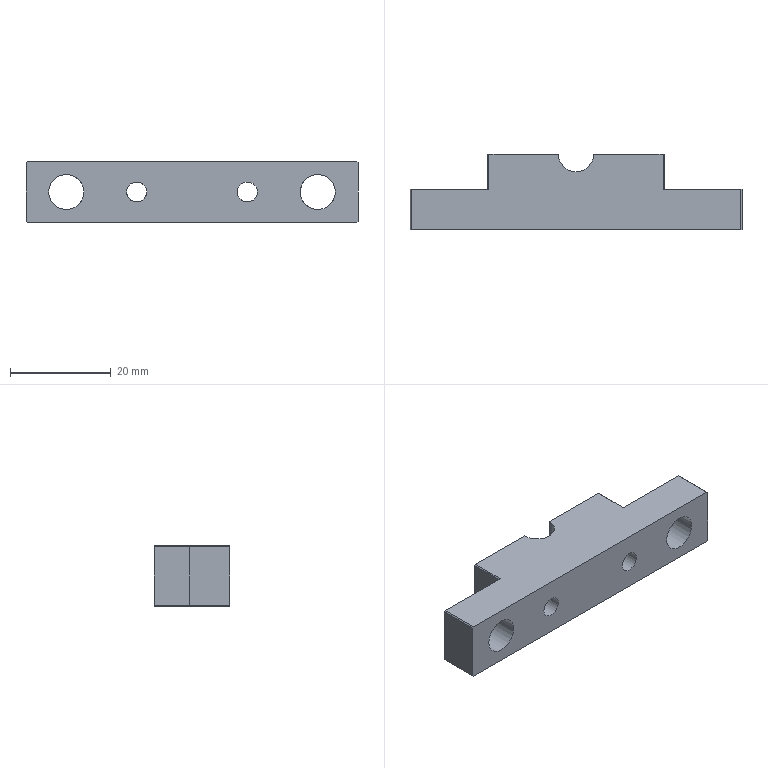Part | NX | 1 solid | 24 faces | box 66 x 15 x 12 mm | volume 8051 mm3 | plane 19 | cylinder 5 | commonest cylinder face diameters 7 x3 4 x2
STEP:
#1=CARTESIAN_POINT('',(36.5,15.,12.));
#2=VERTEX_POINT('',#1);
#3=CARTESIAN_POINT('',(36.5,15.,0.));
#4=VERTEX_POINT('',#3);
#5=CARTESIAN_POINT('',(36.5,15.,12.));
#6=DIRECTION('',(0.,0.,-1.));
#7=VECTOR('',#6,1000.);
#8=LINE('',#5,#7);
#9=EDGE_CURVE('',#2,#4,#8,.T.);
#10=ORIENTED_EDGE('',*,*,#9,.F.);
#11=CARTESIAN_POINT('',(50.3,15.,12.));
#12=VERTEX_POINT('',#11);
#13=CARTESIAN_POINT('',(33.,15.,12.));
#14=DIRECTION('',(1.,0.,0.));
#15=VECTOR('',#14,1000.);
#16=LINE('',#13,#15);
#17=EDGE_CURVE('',#2,#12,#16,.T.);
#18=ORIENTED_EDGE('',*,*,#17,.T.);
#19=CARTESIAN_POINT('',(50.5,15.,11.8));
#20=VERTEX_POINT('',#19);
#21=CARTESIAN_POINT('',(47.65,15.,14.65));
#22=DIRECTION('',(-0.7071,0.,0.7071));
#23=VECTOR('',#22,1000.);
#24=LINE('',#21,#23);
#25=EDGE_CURVE('',#12,#20,#24,.F.);
#26=ORIENTED_EDGE('',*,*,#25,.T.);
#27=CARTESIAN_POINT('',(50.5,15.,0.2));
#28=VERTEX_POINT('',#27);
#29=CARTESIAN_POINT('',(50.5,15.,0.));
#30=DIRECTION('',(0.,0.,-1.));
#31=VECTOR('',#30,1000.);
#32=LINE('',#29,#31);
#33=EDGE_CURVE('',#20,#28,#32,.T.);
#34=ORIENTED_EDGE('',*,*,#33,.T.);
#35=CARTESIAN_POINT('',(50.3,15.,0.));
#36=VERTEX_POINT('',#35);
#37=CARTESIAN_POINT('',(41.65,15.,-8.65));
#38=DIRECTION('',(0.7071,0.,0.7071));
#39=VECTOR('',#38,1000.);
#40=LINE('',#37,#39);
#41=EDGE_CURVE('',#28,#36,#40,.F.);
#42=ORIENTED_EDGE('',*,*,#41,.T.);
#43=CARTESIAN_POINT('',(33.,15.,0.));
#44=DIRECTION('',(-1.,0.,0.));
#45=VECTOR('',#44,1000.);
#46=LINE('',#43,#45);
#47=EDGE_CURVE('',#36,#4,#46,.T.);
#48=ORIENTED_EDGE('',*,*,#47,.T.);
#49=EDGE_LOOP('',(#10,#18,#26,#34,#42,#48));
#50=FACE_BOUND('',#49,.T.);
#51=CARTESIAN_POINT('',(44.,15.,8.));
#52=VERTEX_POINT('',#51);
#53=CARTESIAN_POINT('',(44.,15.,6.));
#54=DIRECTION('',(0.,1.,0.));
#55=DIRECTION('',(0.,0.,1.));
#56=AXIS2_PLACEMENT_3D('',#53,#54,#55);
#57=CIRCLE('',#56,2.);
#58=EDGE_CURVE('',#52,#52,#57,.T.);
#59=ORIENTED_EDGE('',*,*,#58,.F.);
#60=EDGE_LOOP('',(#59));
#61=FACE_BOUND('',#60,.T.);
#62=CARTESIAN_POINT('',(33.,15.,0.));
#63=DIRECTION('',(0.,1.,0.));
#64=DIRECTION('',(0.,0.,1.));
#65=AXIS2_PLACEMENT_3D('',#62,#63,#64);
#66=PLANE('',#65);
#67=ADVANCED_FACE('',(#50,#61),#66,.T.);
#68=CARTESIAN_POINT('',(50.5,8.,11.8));
#69=VERTEX_POINT('',#68);
#70=CARTESIAN_POINT('',(50.5,8.,0.2));
#71=VERTEX_POINT('',#70);
#72=CARTESIAN_POINT('',(50.5,8.,6.));
#73=DIRECTION('',(0.,0.,1.));
#74=VECTOR('',#73,1000.);
#75=LINE('',#72,#74);
#76=EDGE_CURVE('',#69,#71,#75,.F.);
#77=ORIENTED_EDGE('',*,*,#76,.T.);
#78=CARTESIAN_POINT('',(50.5,11.5,0.2));
#79=DIRECTION('',(0.,1.,0.));
#80=VECTOR('',#79,1000.);
#81=LINE('',#78,#80);
#82=EDGE_CURVE('',#71,#28,#81,.T.);
#83=ORIENTED_EDGE('',*,*,#82,.T.);
#84=ORIENTED_EDGE('',*,*,#33,.F.);
#85=CARTESIAN_POINT('',(50.5,11.5,11.8));
#86=DIRECTION('',(0.,-1.,0.));
#87=VECTOR('',#86,1000.);
#88=LINE('',#85,#87);
#89=EDGE_CURVE('',#20,#69,#88,.T.);
#90=ORIENTED_EDGE('',*,*,#89,.T.);
#91=EDGE_LOOP('',(#77,#83,#84,#90));
#92=FACE_BOUND('',#91,.T.);
#93=CARTESIAN_POINT('',(50.5,11.5,6.));
#94=DIRECTION('',(1.,0.,0.));
#95=DIRECTION('',(0.,0.,-1.));
#96=AXIS2_PLACEMENT_3D('',#93,#94,#95);
#97=PLANE('',#96);
#98=ADVANCED_FACE('',(#92),#97,.T.);
#99=ORIENTED_EDGE('',*,*,#58,.T.);
#100=EDGE_LOOP('',(#99));
#101=FACE_BOUND('',#100,.T.);
#102=CARTESIAN_POINT('',(46.,0.,6.));
#103=VERTEX_POINT('',#102);
#104=CARTESIAN_POINT('',(44.,0.,6.));
#105=DIRECTION('',(0.,1.,0.));
#106=DIRECTION('',(1.,0.,0.));
#107=AXIS2_PLACEMENT_3D('',#104,#105,#106);
#108=CIRCLE('',#107,2.);
#109=EDGE_CURVE('',#103,#103,#108,.T.);
#110=ORIENTED_EDGE('',*,*,#109,.F.);
#111=EDGE_LOOP('',(#110));
#112=FACE_BOUND('',#111,.T.);
#113=CARTESIAN_POINT('',(44.,0.,6.));
#114=DIRECTION('',(0.,1.,0.));
#115=DIRECTION('',(1.,0.,0.));
#116=AXIS2_PLACEMENT_3D('',#113,#114,#115);
#117=CYLINDRICAL_SURFACE('',#116,2.);
#118=ADVANCED_FACE('',(#101,#112),#117,.F.);
#119=CARTESIAN_POINT('',(22.,15.,8.));
#120=VERTEX_POINT('',#119);
#121=CARTESIAN_POINT('',(22.,15.,6.));
#122=DIRECTION('',(0.,1.,0.));
#123=DIRECTION('',(0.,0.,1.));
#124=AXIS2_PLACEMENT_3D('',#121,#122,#123);
#125=CIRCLE('',#124,2.);
#126=EDGE_CURVE('',#120,#120,#125,.T.);
#127=ORIENTED_EDGE('',*,*,#126,.T.);
#128=EDGE_LOOP('',(#127));
#129=FACE_BOUND('',#128,.T.);
#130=CARTESIAN_POINT('',(24.,0.,6.));
#131=VERTEX_POINT('',#130);
#132=CARTESIAN_POINT('',(22.,0.,6.));
#133=DIRECTION('',(0.,1.,0.));
#134=DIRECTION('',(1.,0.,0.));
#135=AXIS2_PLACEMENT_3D('',#132,#133,#134);
#136=CIRCLE('',#135,2.);
#137=EDGE_CURVE('',#131,#131,#136,.T.);
#138=ORIENTED_EDGE('',*,*,#137,.F.);
#139=EDGE_LOOP('',(#138));
#140=FACE_BOUND('',#139,.T.);
#141=CARTESIAN_POINT('',(22.,0.,6.));
#142=DIRECTION('',(0.,1.,0.));
#143=DIRECTION('',(1.,0.,0.));
#144=AXIS2_PLACEMENT_3D('',#141,#142,#143);
#145=CYLINDRICAL_SURFACE('',#144,2.);
#146=ADVANCED_FACE('',(#129,#140),#145,.F.);
#147=CARTESIAN_POINT('',(15.5,15.,11.8));
#148=VERTEX_POINT('',#147);
#149=CARTESIAN_POINT('',(15.5,15.,0.2));
#150=VERTEX_POINT('',#149);
#151=CARTESIAN_POINT('',(15.5,15.,0.));
#152=DIRECTION('',(0.,0.,1.));
#153=VECTOR('',#152,1000.);
#154=LINE('',#151,#153);
#155=EDGE_CURVE('',#148,#150,#154,.F.);
#156=ORIENTED_EDGE('',*,*,#155,.T.);
#157=CARTESIAN_POINT('',(15.5,8.,0.2));
#158=VERTEX_POINT('',#157);
#159=CARTESIAN_POINT('',(15.5,11.5,0.2));
#160=DIRECTION('',(0.,-1.,0.));
#161=VECTOR('',#160,1000.);
#162=LINE('',#159,#161);
#163=EDGE_CURVE('',#150,#158,#162,.T.);
#164=ORIENTED_EDGE('',*,*,#163,.T.);
#165=CARTESIAN_POINT('',(15.5,8.,11.8));
#166=VERTEX_POINT('',#165);
#167=CARTESIAN_POINT('',(15.5,8.,6.));
#168=DIRECTION('',(0.,0.,-1.));
#169=VECTOR('',#168,1000.);
#170=LINE('',#167,#169);
#171=EDGE_CURVE('',#158,#166,#170,.F.);
#172=ORIENTED_EDGE('',*,*,#171,.T.);
#173=CARTESIAN_POINT('',(15.5,11.5,11.8));
#174=DIRECTION('',(0.,1.,0.));
#175=VECTOR('',#174,1000.);
#176=LINE('',#173,#175);
#177=EDGE_CURVE('',#166,#148,#176,.T.);
#178=ORIENTED_EDGE('',*,*,#177,.T.);
#179=EDGE_LOOP('',(#156,#164,#172,#178));
#180=FACE_BOUND('',#179,.T.);
#181=CARTESIAN_POINT('',(15.5,11.5,6.));
#182=DIRECTION('',(-1.,0.,0.));
#183=DIRECTION('',(0.,0.,1.));
#184=AXIS2_PLACEMENT_3D('',#181,#182,#183);
#185=PLANE('',#184);
#186=ADVANCED_FACE('',(#180),#185,.T.);
#187=CARTESIAN_POINT('',(29.5,15.,12.));
#188=VERTEX_POINT('',#187);
#189=CARTESIAN_POINT('',(33.,15.,12.));
#190=DIRECTION('',(0.,0.,-1.));
#191=DIRECTION('',(1.,0.,0.));
#192=AXIS2_PLACEMENT_3D('',#189,#190,#191);
#193=CIRCLE('',#192,3.5);
#194=EDGE_CURVE('',#2,#188,#193,.T.);
#195=ORIENTED_EDGE('',*,*,#194,.T.);
#196=CARTESIAN_POINT('',(15.7,15.,12.));
#197=VERTEX_POINT('',#196);
#198=CARTESIAN_POINT('',(33.,15.,12.));
#199=DIRECTION('',(1.,0.,0.));
#200=VECTOR('',#199,1000.);
#201=LINE('',#198,#200);
#202=EDGE_CURVE('',#197,#188,#201,.T.);
#203=ORIENTED_EDGE('',*,*,#202,.F.);
#204=CARTESIAN_POINT('',(15.7,8.,12.));
#205=VERTEX_POINT('',#204);
#206=CARTESIAN_POINT('',(15.7,7.5,12.));
#207=DIRECTION('',(0.,-1.,0.));
#208=VECTOR('',#207,1000.);
#209=LINE('',#206,#208);
#210=EDGE_CURVE('',#197,#205,#209,.T.);
#211=ORIENTED_EDGE('',*,*,#210,.T.);
#212=CARTESIAN_POINT('',(0.2,8.,12.));
#213=VERTEX_POINT('',#212);
#214=CARTESIAN_POINT('',(33.,8.,12.));
#215=DIRECTION('',(1.,0.,0.));
#216=VECTOR('',#215,1000.);
#217=LINE('',#214,#216);
#218=EDGE_CURVE('',#213,#205,#217,.T.);
#219=ORIENTED_EDGE('',*,*,#218,.F.);
#220=CARTESIAN_POINT('',(0.2,0.,12.));
#221=VERTEX_POINT('',#220);
#222=CARTESIAN_POINT('',(0.2,7.5,12.));
#223=DIRECTION('',(0.,-1.,0.));
#224=VECTOR('',#223,1000.);
#225=LINE('',#222,#224);
#226=EDGE_CURVE('',#213,#221,#225,.T.);
#227=ORIENTED_EDGE('',*,*,#226,.T.);
#228=CARTESIAN_POINT('',(65.8,0.,12.));
#229=VERTEX_POINT('',#228);
#230=CARTESIAN_POINT('',(33.,0.,12.));
#231=DIRECTION('',(-1.,0.,0.));
#232=VECTOR('',#231,1000.);
#233=LINE('',#230,#232);
#234=EDGE_CURVE('',#229,#221,#233,.T.);
#235=ORIENTED_EDGE('',*,*,#234,.F.);
#236=CARTESIAN_POINT('',(65.8,8.,12.));
#237=VERTEX_POINT('',#236);
#238=CARTESIAN_POINT('',(65.8,7.5,12.));
#239=DIRECTION('',(0.,1.,0.));
#240=VECTOR('',#239,1000.);
#241=LINE('',#238,#240);
#242=EDGE_CURVE('',#229,#237,#241,.T.);
#243=ORIENTED_EDGE('',*,*,#242,.T.);
#244=CARTESIAN_POINT('',(50.3,8.,12.));
#245=VERTEX_POINT('',#244);
#246=CARTESIAN_POINT('',(33.,8.,12.));
#247=DIRECTION('',(1.,0.,0.));
#248=VECTOR('',#247,1000.);
#249=LINE('',#246,#248);
#250=EDGE_CURVE('',#245,#237,#249,.T.);
#251=ORIENTED_EDGE('',*,*,#250,.F.);
#252=CARTESIAN_POINT('',(50.3,7.5,12.));
#253=DIRECTION('',(0.,1.,0.));
#254=VECTOR('',#253,1000.);
#255=LINE('',#252,#254);
#256=EDGE_CURVE('',#245,#12,#255,.T.);
#257=ORIENTED_EDGE('',*,*,#256,.T.);
#258=ORIENTED_EDGE('',*,*,#17,.F.);
#259=EDGE_LOOP('',(#195,#203,#211,#219,#227,#235,#243,#251,#257,#258));
#260=FACE_BOUND('',#259,.T.);
#261=CARTESIAN_POINT('',(33.,7.5,12.));
#262=DIRECTION('',(0.,0.,1.));
#263=DIRECTION('',(1.,0.,0.));
#264=AXIS2_PLACEMENT_3D('',#261,#262,#263);
#265=PLANE('',#264);
#266=ADVANCED_FACE('',(#260),#265,.T.);
#267=CARTESIAN_POINT('',(29.5,15.,0.));
#268=VERTEX_POINT('',#267);
#269=CARTESIAN_POINT('',(33.,15.,0.));
#270=DIRECTION('',(0.,0.,-1.));
#271=DIRECTION('',(-1.,0.,0.));
#272=AXIS2_PLACEMENT_3D('',#269,#270,#271);
#273=CIRCLE('',#272,3.5);
#274=EDGE_CURVE('',#4,#268,#273,.T.);
#275=ORIENTED_EDGE('',*,*,#274,.F.);
#276=ORIENTED_EDGE('',*,*,#47,.F.);
#277=CARTESIAN_POINT('',(50.3,8.,0.));
#278=VERTEX_POINT('',#277);
#279=CARTESIAN_POINT('',(50.3,7.5,0.));
#280=DIRECTION('',(0.,-1.,0.));
#281=VECTOR('',#280,1000.);
#282=LINE('',#279,#281);
#283=EDGE_CURVE('',#36,#278,#282,.T.);
#284=ORIENTED_EDGE('',*,*,#283,.T.);
#285=CARTESIAN_POINT('',(65.8,8.,0.));
#286=VERTEX_POINT('',#285);
#287=CARTESIAN_POINT('',(33.,8.,0.));
#288=DIRECTION('',(-1.,0.,0.));
#289=VECTOR('',#288,1000.);
#290=LINE('',#287,#289);
#291=EDGE_CURVE('',#278,#286,#290,.F.);
#292=ORIENTED_EDGE('',*,*,#291,.T.);
#293=CARTESIAN_POINT('',(65.8,0.,0.));
#294=VERTEX_POINT('',#293);
#295=CARTESIAN_POINT('',(65.8,7.5,0.));
#296=DIRECTION('',(0.,-1.,0.));
#297=VECTOR('',#296,1000.);
#298=LINE('',#295,#297);
#299=EDGE_CURVE('',#286,#294,#298,.T.);
#300=ORIENTED_EDGE('',*,*,#299,.T.);
#301=CARTESIAN_POINT('',(0.2,0.,0.));
#302=VERTEX_POINT('',#301);
#303=CARTESIAN_POINT('',(33.,0.,0.));
#304=DIRECTION('',(1.,0.,0.));
#305=VECTOR('',#304,1000.);
#306=LINE('',#303,#305);
#307=EDGE_CURVE('',#302,#294,#306,.T.);
#308=ORIENTED_EDGE('',*,*,#307,.F.);
#309=CARTESIAN_POINT('',(0.2,8.,0.));
#310=VERTEX_POINT('',#309);
#311=CARTESIAN_POINT('',(0.2,7.5,0.));
#312=DIRECTION('',(0.,1.,0.));
#313=VECTOR('',#312,1000.);
#314=LINE('',#311,#313);
#315=EDGE_CURVE('',#302,#310,#314,.T.);
#316=ORIENTED_EDGE('',*,*,#315,.T.);
#317=CARTESIAN_POINT('',(15.7,8.,0.));
#318=VERTEX_POINT('',#317);
#319=CARTESIAN_POINT('',(33.,8.,0.));
#320=DIRECTION('',(-1.,0.,0.));
#321=VECTOR('',#320,1000.);
#322=LINE('',#319,#321);
#323=EDGE_CURVE('',#310,#318,#322,.F.);
#324=ORIENTED_EDGE('',*,*,#323,.T.);
#325=CARTESIAN_POINT('',(15.7,15.,0.));
#326=VERTEX_POINT('',#325);
#327=CARTESIAN_POINT('',(15.7,7.5,0.));
#328=DIRECTION('',(0.,1.,0.));
#329=VECTOR('',#328,1000.);
#330=LINE('',#327,#329);
#331=EDGE_CURVE('',#318,#326,#330,.T.);
#332=ORIENTED_EDGE('',*,*,#331,.T.);
#333=CARTESIAN_POINT('',(33.,15.,0.));
#334=DIRECTION('',(-1.,0.,0.));
#335=VECTOR('',#334,1000.);
#336=LINE('',#333,#335);
#337=EDGE_CURVE('',#268,#326,#336,.T.);
#338=ORIENTED_EDGE('',*,*,#337,.F.);
#339=EDGE_LOOP('',(#275,#276,#284,#292,#300,#308,#316,#324,#332,#338));
#340=FACE_BOUND('',#339,.T.);
#341=CARTESIAN_POINT('',(33.,7.5,0.));
#342=DIRECTION('',(0.,0.,-1.));
#343=DIRECTION('',(-1.,0.,0.));
#344=AXIS2_PLACEMENT_3D('',#341,#342,#343);
#345=PLANE('',#344);
#346=ADVANCED_FACE('',(#340),#345,.T.);
#347=CARTESIAN_POINT('',(29.5,15.,12.));
#348=DIRECTION('',(0.,0.,-1.));
#349=VECTOR('',#348,1000.);
#350=LINE('',#347,#349);
#351=EDGE_CURVE('',#268,#188,#350,.F.);
#352=ORIENTED_EDGE('',*,*,#351,.F.);
#353=ORIENTED_EDGE('',*,*,#337,.T.);
#354=CARTESIAN_POINT('',(24.35,15.,-8.65));
#355=DIRECTION('',(0.7071,0.,-0.7071));
#356=VECTOR('',#355,1000.);
#357=LINE('',#354,#356);
#358=EDGE_CURVE('',#326,#150,#357,.F.);
#359=ORIENTED_EDGE('',*,*,#358,.T.);
#360=ORIENTED_EDGE('',*,*,#155,.F.);
#361=CARTESIAN_POINT('',(18.35,15.,14.65));
#362=DIRECTION('',(-0.7071,0.,-0.7071));
#363=VECTOR('',#362,1000.);
#364=LINE('',#361,#363);
#365=EDGE_CURVE('',#148,#197,#364,.F.);
#366=ORIENTED_EDGE('',*,*,#365,.T.);
#367=ORIENTED_EDGE('',*,*,#202,.T.);
#368=EDGE_LOOP('',(#352,#353,#359,#360,#366,#367));
#369=FACE_BOUND('',#368,.T.);
#370=ORIENTED_EDGE('',*,*,#126,.F.);
#371=EDGE_LOOP('',(#370));
#372=FACE_BOUND('',#371,.T.);
#373=CARTESIAN_POINT('',(33.,15.,0.));
#374=DIRECTION('',(0.,1.,0.));
#375=DIRECTION('',(0.,0.,1.));
#376=AXIS2_PLACEMENT_3D('',#373,#374,#375);
#377=PLANE('',#376);
#378=ADVANCED_FACE('',(#369,#372),#377,.T.);
#379=CARTESIAN_POINT('',(66.,8.,11.8));
#380=VERTEX_POINT('',#379);
#381=CARTESIAN_POINT('',(66.,8.,0.2));
#382=VERTEX_POINT('',#381);
#383=CARTESIAN_POINT('',(66.,8.,0.));
#384=DIRECTION('',(0.,0.,-1.));
#385=VECTOR('',#384,1000.);
#386=LINE('',#383,#385);
#387=EDGE_CURVE('',#380,#382,#386,.T.);
#388=ORIENTED_EDGE('',*,*,#387,.T.);
#389=CARTESIAN_POINT('',(66.,8.,0.2));
#390=DIRECTION('',(0.7071,0.,0.7071));
#391=VECTOR('',#390,1000.);
#392=LINE('',#389,#391);
#393=EDGE_CURVE('',#382,#286,#392,.F.);
#394=ORIENTED_EDGE('',*,*,#393,.T.);
#395=ORIENTED_EDGE('',*,*,#291,.F.);
#396=CARTESIAN_POINT('',(44.65,8.,-5.65));
#397=DIRECTION('',(-0.7071,0.,-0.7071));
#398=VECTOR('',#397,1000.);
#399=LINE('',#396,#398);
#400=EDGE_CURVE('',#278,#71,#399,.F.);
#401=ORIENTED_EDGE('',*,*,#400,.T.);
#402=ORIENTED_EDGE('',*,*,#76,.F.);
#403=CARTESIAN_POINT('',(44.65,8.,17.65));
#404=DIRECTION('',(0.7071,0.,-0.7071));
#405=VECTOR('',#404,1000.);
#406=LINE('',#403,#405);
#407=EDGE_CURVE('',#69,#245,#406,.F.);
#408=ORIENTED_EDGE('',*,*,#407,.T.);
#409=ORIENTED_EDGE('',*,*,#250,.T.);
#410=CARTESIAN_POINT('',(66.,8.,11.8));
#411=DIRECTION('',(-0.7071,0.,0.7071));
#412=VECTOR('',#411,1000.);
#413=LINE('',#410,#412);
#414=EDGE_CURVE('',#237,#380,#413,.F.);
#415=ORIENTED_EDGE('',*,*,#414,.T.);
#416=EDGE_LOOP('',(#388,#394,#395,#401,#402,#408,#409,#415));
#417=FACE_BOUND('',#416,.T.);
#418=CARTESIAN_POINT('',(58.,8.,2.5));
#419=VERTEX_POINT('',#418);
#420=CARTESIAN_POINT('',(58.,8.,6.));
#421=DIRECTION('',(0.,-1.,0.));
#422=DIRECTION('',(0.,0.,-1.));
#423=AXIS2_PLACEMENT_3D('',#420,#421,#422);
#424=CIRCLE('',#423,3.5);
#425=EDGE_CURVE('',#419,#419,#424,.T.);
#426=ORIENTED_EDGE('',*,*,#425,.T.);
#427=EDGE_LOOP('',(#426));
#428=FACE_BOUND('',#427,.T.);
#429=CARTESIAN_POINT('',(33.,8.,6.));
#430=DIRECTION('',(0.,-1.,0.));
#431=DIRECTION('',(0.,0.,-1.));
#432=AXIS2_PLACEMENT_3D('',#429,#430,#431);
#433=PLANE('',#432);
#434=ADVANCED_FACE('',(#417,#428),#433,.F.);
#435=CARTESIAN_POINT('',(66.,0.,0.2));
#436=VERTEX_POINT('',#435);
#437=CARTESIAN_POINT('',(66.,0.,11.8));
#438=VERTEX_POINT('',#437);
#439=CARTESIAN_POINT('',(66.,0.,0.));
#440=DIRECTION('',(0.,0.,1.));
#441=VECTOR('',#440,1000.);
#442=LINE('',#439,#441);
#443=EDGE_CURVE('',#436,#438,#442,.T.);
#444=ORIENTED_EDGE('',*,*,#443,.F.);
#445=CARTESIAN_POINT('',(66.,7.5,0.2));
#446=DIRECTION('',(0.,1.,0.));
#447=VECTOR('',#446,1000.);
#448=LINE('',#445,#447);
#449=EDGE_CURVE('',#436,#382,#448,.T.);
#450=ORIENTED_EDGE('',*,*,#449,.T.);
#451=ORIENTED_EDGE('',*,*,#387,.F.);
#452=CARTESIAN_POINT('',(66.,7.5,11.8));
#453=DIRECTION('',(0.,-1.,0.));
#454=VECTOR('',#453,1000.);
#455=LINE('',#452,#454);
#456=EDGE_CURVE('',#380,#438,#455,.T.);
#457=ORIENTED_EDGE('',*,*,#456,.T.);
#458=EDGE_LOOP('',(#444,#450,#451,#457));
#459=FACE_BOUND('',#458,.T.);
#460=CARTESIAN_POINT('',(66.,7.5,0.));
#461=DIRECTION('',(1.,0.,0.));
#462=DIRECTION('',(0.,0.,-1.));
#463=AXIS2_PLACEMENT_3D('',#460,#461,#462);
#464=PLANE('',#463);
#465=ADVANCED_FACE('',(#459),#464,.T.);
#466=CARTESIAN_POINT('',(0.,8.,0.2));
#467=VERTEX_POINT('',#466);
#468=CARTESIAN_POINT('',(0.,8.,11.8));
#469=VERTEX_POINT('',#468);
#470=CARTESIAN_POINT('',(0.,8.,0.));
#471=DIRECTION('',(0.,0.,1.));
#472=VECTOR('',#471,1000.);
#473=LINE('',#470,#472);
#474=EDGE_CURVE('',#467,#469,#473,.T.);
#475=ORIENTED_EDGE('',*,*,#474,.F.);
#476=CARTESIAN_POINT('',(0.,0.,0.2));
#477=VERTEX_POINT('',#476);
#478=CARTESIAN_POINT('',(0.,7.5,0.2));
#479=DIRECTION('',(0.,-1.,0.));
#480=VECTOR('',#479,1000.);
#481=LINE('',#478,#480);
#482=EDGE_CURVE('',#467,#477,#481,.T.);
#483=ORIENTED_EDGE('',*,*,#482,.T.);
#484=CARTESIAN_POINT('',(0.,0.,11.8));
#485=VERTEX_POINT('',#484);
#486=CARTESIAN_POINT('',(0.,0.,0.));
#487=DIRECTION('',(0.,0.,1.));
#488=VECTOR('',#487,1000.);
#489=LINE('',#486,#488);
#490=EDGE_CURVE('',#477,#485,#489,.T.);
#491=ORIENTED_EDGE('',*,*,#490,.T.);
#492=CARTESIAN_POINT('',(0.,7.5,11.8));
#493=DIRECTION('',(0.,1.,0.));
#494=VECTOR('',#493,1000.);
#495=LINE('',#492,#494);
#496=EDGE_CURVE('',#485,#469,#495,.T.);
#497=ORIENTED_EDGE('',*,*,#496,.T.);
#498=EDGE_LOOP('',(#475,#483,#491,#497));
#499=FACE_BOUND('',#498,.T.);
#500=CARTESIAN_POINT('',(0.,7.5,0.));
#501=DIRECTION('',(-1.,0.,0.));
#502=DIRECTION('',(0.,0.,1.));
#503=AXIS2_PLACEMENT_3D('',#500,#501,#502);
#504=PLANE('',#503);
#505=ADVANCED_FACE('',(#499),#504,.T.);
#506=ORIENTED_EDGE('',*,*,#425,.F.);
#507=EDGE_LOOP('',(#506));
#508=FACE_BOUND('',#507,.T.);
#509=CARTESIAN_POINT('',(61.5,0.,6.));
#510=VERTEX_POINT('',#509);
#511=CARTESIAN_POINT('',(58.,0.,6.));
#512=DIRECTION('',(0.,1.,0.));
#513=DIRECTION('',(1.,0.,0.));
#514=AXIS2_PLACEMENT_3D('',#511,#512,#513);
#515=CIRCLE('',#514,3.5);
#516=EDGE_CURVE('',#510,#510,#515,.T.);
#517=ORIENTED_EDGE('',*,*,#516,.F.);
#518=EDGE_LOOP('',(#517));
#519=FACE_BOUND('',#518,.T.);
#520=CARTESIAN_POINT('',(58.,0.,6.));
#521=DIRECTION('',(0.,1.,0.));
#522=DIRECTION('',(1.,0.,0.));
#523=AXIS2_PLACEMENT_3D('',#520,#521,#522);
#524=CYLINDRICAL_SURFACE('',#523,3.5);
#525=ADVANCED_FACE('',(#508,#519),#524,.F.);
#526=CARTESIAN_POINT('',(11.5,0.,6.));
#527=VERTEX_POINT('',#526);
#528=CARTESIAN_POINT('',(8.,0.,6.));
#529=DIRECTION('',(0.,1.,0.));
#530=DIRECTION('',(1.,0.,0.));
#531=AXIS2_PLACEMENT_3D('',#528,#529,#530);
#532=CIRCLE('',#531,3.5);
#533=EDGE_CURVE('',#527,#527,#532,.T.);
#534=ORIENTED_EDGE('',*,*,#533,.T.);
#535=EDGE_LOOP('',(#534));
#536=FACE_BOUND('',#535,.T.);
#537=ORIENTED_EDGE('',*,*,#109,.T.);
#538=EDGE_LOOP('',(#537));
#539=FACE_BOUND('',#538,.T.);
#540=ORIENTED_EDGE('',*,*,#137,.T.);
#541=EDGE_LOOP('',(#540));
#542=FACE_BOUND('',#541,.T.);
#543=ORIENTED_EDGE('',*,*,#516,.T.);
#544=EDGE_LOOP('',(#543));
#545=FACE_BOUND('',#544,.T.);
#546=ORIENTED_EDGE('',*,*,#307,.T.);
#547=CARTESIAN_POINT('',(49.4,0.,-16.4));
#548=DIRECTION('',(-0.7071,0.,-0.7071));
#549=VECTOR('',#548,1000.);
#550=LINE('',#547,#549);
#551=EDGE_CURVE('',#294,#436,#550,.F.);
#552=ORIENTED_EDGE('',*,*,#551,.T.);
#553=ORIENTED_EDGE('',*,*,#443,.T.);
#554=CARTESIAN_POINT('',(55.4,0.,22.4));
#555=DIRECTION('',(0.7071,0.,-0.7071));
#556=VECTOR('',#555,1000.);
#557=LINE('',#554,#556);
#558=EDGE_CURVE('',#438,#229,#557,.F.);
#559=ORIENTED_EDGE('',*,*,#558,.T.);
#560=ORIENTED_EDGE('',*,*,#234,.T.);
#561=CARTESIAN_POINT('',(10.6,0.,22.4));
#562=DIRECTION('',(0.7071,0.,0.7071));
#563=VECTOR('',#562,1000.);
#564=LINE('',#561,#563);
#565=EDGE_CURVE('',#221,#485,#564,.F.);
#566=ORIENTED_EDGE('',*,*,#565,.T.);
#567=ORIENTED_EDGE('',*,*,#490,.F.);
#568=CARTESIAN_POINT('',(16.6,0.,-16.4));
#569=DIRECTION('',(-0.7071,0.,0.7071));
#570=VECTOR('',#569,1000.);
#571=LINE('',#568,#570);
#572=EDGE_CURVE('',#477,#302,#571,.F.);
#573=ORIENTED_EDGE('',*,*,#572,.T.);
#574=EDGE_LOOP('',(#546,#552,#553,#559,#560,#566,#567,#573));
#575=FACE_BOUND('',#574,.T.);
#576=CARTESIAN_POINT('',(33.,0.,0.));
#577=DIRECTION('',(0.,-1.,0.));
#578=DIRECTION('',(0.,0.,-1.));
#579=AXIS2_PLACEMENT_3D('',#576,#577,#578);
#580=PLANE('',#579);
#581=ADVANCED_FACE('',(#536,#539,#542,#545,#575),#580,.T.);
#582=CARTESIAN_POINT('',(8.,8.,2.5));
#583=VERTEX_POINT('',#582);
#584=CARTESIAN_POINT('',(8.,8.,6.));
#585=DIRECTION('',(0.,-1.,0.));
#586=DIRECTION('',(0.,0.,-1.));
#587=AXIS2_PLACEMENT_3D('',#584,#585,#586);
#588=CIRCLE('',#587,3.5);
#589=EDGE_CURVE('',#583,#583,#588,.F.);
#590=ORIENTED_EDGE('',*,*,#589,.T.);
#591=EDGE_LOOP('',(#590));
#592=FACE_BOUND('',#591,.T.);
#593=ORIENTED_EDGE('',*,*,#533,.F.);
#594=EDGE_LOOP('',(#593));
#595=FACE_BOUND('',#594,.T.);
#596=CARTESIAN_POINT('',(8.,0.,6.));
#597=DIRECTION('',(0.,1.,0.));
#598=DIRECTION('',(1.,0.,0.));
#599=AXIS2_PLACEMENT_3D('',#596,#597,#598);
#600=CYLINDRICAL_SURFACE('',#599,3.5);
#601=ADVANCED_FACE('',(#592,#595),#600,.F.);
#602=ORIENTED_EDGE('',*,*,#323,.F.);
#603=CARTESIAN_POINT('',(0.,8.,0.2));
#604=DIRECTION('',(0.7071,0.,-0.7071));
#605=VECTOR('',#604,1000.);
#606=LINE('',#603,#605);
#607=EDGE_CURVE('',#310,#467,#606,.F.);
#608=ORIENTED_EDGE('',*,*,#607,.T.);
#609=ORIENTED_EDGE('',*,*,#474,.T.);
#610=CARTESIAN_POINT('',(0.,8.,11.8));
#611=DIRECTION('',(-0.7071,0.,-0.7071));
#612=VECTOR('',#611,1000.);
#613=LINE('',#610,#612);
#614=EDGE_CURVE('',#469,#213,#613,.F.);
#615=ORIENTED_EDGE('',*,*,#614,.T.);
#616=ORIENTED_EDGE('',*,*,#218,.T.);
#617=CARTESIAN_POINT('',(21.35,8.,17.65));
#618=DIRECTION('',(0.7071,0.,0.7071));
#619=VECTOR('',#618,1000.);
#620=LINE('',#617,#619);
#621=EDGE_CURVE('',#205,#166,#620,.F.);
#622=ORIENTED_EDGE('',*,*,#621,.T.);
#623=ORIENTED_EDGE('',*,*,#171,.F.);
#624=CARTESIAN_POINT('',(21.35,8.,-5.65));
#625=DIRECTION('',(-0.7071,0.,0.7071));
#626=VECTOR('',#625,1000.);
#627=LINE('',#624,#626);
#628=EDGE_CURVE('',#158,#318,#627,.F.);
#629=ORIENTED_EDGE('',*,*,#628,.T.);
#630=EDGE_LOOP('',(#602,#608,#609,#615,#616,#622,#623,#629));
#631=FACE_BOUND('',#630,.T.);
#632=ORIENTED_EDGE('',*,*,#589,.F.);
#633=EDGE_LOOP('',(#632));
#634=FACE_BOUND('',#633,.T.);
#635=CARTESIAN_POINT('',(33.,8.,6.));
#636=DIRECTION('',(0.,-1.,0.));
#637=DIRECTION('',(0.,0.,-1.));
#638=AXIS2_PLACEMENT_3D('',#635,#636,#637);
#639=PLANE('',#638);
#640=ADVANCED_FACE('',(#631,#634),#639,.F.);
#641=ORIENTED_EDGE('',*,*,#551,.F.);
#642=ORIENTED_EDGE('',*,*,#299,.F.);
#643=ORIENTED_EDGE('',*,*,#393,.F.);
#644=ORIENTED_EDGE('',*,*,#449,.F.);
#645=EDGE_LOOP('',(#641,#642,#643,#644));
#646=FACE_BOUND('',#645,.T.);
#647=CARTESIAN_POINT('',(66.,7.5,0.2));
#648=DIRECTION('',(-0.7071,0.,0.7071));
#649=DIRECTION('',(0.,1.,0.));
#650=AXIS2_PLACEMENT_3D('',#647,#648,#649);
#651=PLANE('',#650);
#652=ADVANCED_FACE('',(#646),#651,.F.);
#653=ORIENTED_EDGE('',*,*,#414,.F.);
#654=ORIENTED_EDGE('',*,*,#242,.F.);
#655=ORIENTED_EDGE('',*,*,#558,.F.);
#656=ORIENTED_EDGE('',*,*,#456,.F.);
#657=EDGE_LOOP('',(#653,#654,#655,#656));
#658=FACE_BOUND('',#657,.T.);
#659=CARTESIAN_POINT('',(66.,7.5,11.8));
#660=DIRECTION('',(-0.7071,0.,-0.7071));
#661=DIRECTION('',(0.,-1.,0.));
#662=AXIS2_PLACEMENT_3D('',#659,#660,#661);
#663=PLANE('',#662);
#664=ADVANCED_FACE('',(#658),#663,.F.);
#665=ORIENTED_EDGE('',*,*,#400,.F.);
#666=ORIENTED_EDGE('',*,*,#283,.F.);
#667=ORIENTED_EDGE('',*,*,#41,.F.);
#668=ORIENTED_EDGE('',*,*,#82,.F.);
#669=EDGE_LOOP('',(#665,#666,#667,#668));
#670=FACE_BOUND('',#669,.T.);
#671=CARTESIAN_POINT('',(50.5,11.5,0.2));
#672=DIRECTION('',(-0.7071,0.,0.7071));
#673=DIRECTION('',(0.,1.,0.));
#674=AXIS2_PLACEMENT_3D('',#671,#672,#673);
#675=PLANE('',#674);
#676=ADVANCED_FACE('',(#670),#675,.F.);
#677=ORIENTED_EDGE('',*,*,#25,.F.);
#678=ORIENTED_EDGE('',*,*,#256,.F.);
#679=ORIENTED_EDGE('',*,*,#407,.F.);
#680=ORIENTED_EDGE('',*,*,#89,.F.);
#681=EDGE_LOOP('',(#677,#678,#679,#680));
#682=FACE_BOUND('',#681,.T.);
#683=CARTESIAN_POINT('',(50.5,11.5,11.8));
#684=DIRECTION('',(-0.7071,0.,-0.7071));
#685=DIRECTION('',(0.,-1.,0.));
#686=AXIS2_PLACEMENT_3D('',#683,#684,#685);
#687=PLANE('',#686);
#688=ADVANCED_FACE('',(#682),#687,.F.);
#689=ORIENTED_EDGE('',*,*,#358,.F.);
#690=ORIENTED_EDGE('',*,*,#331,.F.);
#691=ORIENTED_EDGE('',*,*,#628,.F.);
#692=ORIENTED_EDGE('',*,*,#163,.F.);
#693=EDGE_LOOP('',(#689,#690,#691,#692));
#694=FACE_BOUND('',#693,.T.);
#695=CARTESIAN_POINT('',(15.5,11.5,0.2));
#696=DIRECTION('',(0.7071,0.,0.7071));
#697=DIRECTION('',(0.,-1.,0.));
#698=AXIS2_PLACEMENT_3D('',#695,#696,#697);
#699=PLANE('',#698);
#700=ADVANCED_FACE('',(#694),#699,.F.);
#701=ORIENTED_EDGE('',*,*,#621,.F.);
#702=ORIENTED_EDGE('',*,*,#210,.F.);
#703=ORIENTED_EDGE('',*,*,#365,.F.);
#704=ORIENTED_EDGE('',*,*,#177,.F.);
#705=EDGE_LOOP('',(#701,#702,#703,#704));
#706=FACE_BOUND('',#705,.T.);
#707=CARTESIAN_POINT('',(15.5,11.5,11.8));
#708=DIRECTION('',(0.7071,0.,-0.7071));
#709=DIRECTION('',(0.,1.,0.));
#710=AXIS2_PLACEMENT_3D('',#707,#708,#709);
#711=PLANE('',#710);
#712=ADVANCED_FACE('',(#706),#711,.F.);
#713=ORIENTED_EDGE('',*,*,#607,.F.);
#714=ORIENTED_EDGE('',*,*,#315,.F.);
#715=ORIENTED_EDGE('',*,*,#572,.F.);
#716=ORIENTED_EDGE('',*,*,#482,.F.);
#717=EDGE_LOOP('',(#713,#714,#715,#716));
#718=FACE_BOUND('',#717,.T.);
#719=CARTESIAN_POINT('',(0.,7.5,0.2));
#720=DIRECTION('',(0.7071,0.,0.7071));
#721=DIRECTION('',(0.,-1.,0.));
#722=AXIS2_PLACEMENT_3D('',#719,#720,#721);
#723=PLANE('',#722);
#724=ADVANCED_FACE('',(#718),#723,.F.);
#725=ORIENTED_EDGE('',*,*,#565,.F.);
#726=ORIENTED_EDGE('',*,*,#226,.F.);
#727=ORIENTED_EDGE('',*,*,#614,.F.);
#728=ORIENTED_EDGE('',*,*,#496,.F.);
#729=EDGE_LOOP('',(#725,#726,#727,#728));
#730=FACE_BOUND('',#729,.T.);
#731=CARTESIAN_POINT('',(0.,7.5,11.8));
#732=DIRECTION('',(0.7071,0.,-0.7071));
#733=DIRECTION('',(0.,1.,0.));
#734=AXIS2_PLACEMENT_3D('',#731,#732,#733);
#735=PLANE('',#734);
#736=ADVANCED_FACE('',(#730),#735,.F.);
#737=ORIENTED_EDGE('',*,*,#9,.T.);
#738=ORIENTED_EDGE('',*,*,#274,.T.);
#739=ORIENTED_EDGE('',*,*,#351,.T.);
#740=ORIENTED_EDGE('',*,*,#194,.F.);
#741=EDGE_LOOP('',(#737,#738,#739,#740));
#742=FACE_BOUND('',#741,.T.);
#743=CARTESIAN_POINT('',(33.,15.,12.));
#744=DIRECTION('',(0.,0.,-1.));
#745=DIRECTION('',(1.,0.,0.));
#746=AXIS2_PLACEMENT_3D('',#743,#744,#745);
#747=CYLINDRICAL_SURFACE('',#746,3.5);
#748=ADVANCED_FACE('',(#742),#747,.F.);
#749=CLOSED_SHELL('',(#67,#98,#118,#146,#186,#266,#346,#378,#434,#465,#505,#525,#581,#601,#640,#652,#664,#676,#688,#700,#712,#724,#736,#748));
#750=MANIFOLD_SOLID_BREP('',#749);
#751=(LENGTH_UNIT()NAMED_UNIT(*)SI_UNIT(.MILLI.,.METRE.));
#752=UNCERTAINTY_MEASURE_WITH_UNIT(LENGTH_MEASURE(0.00001),#751,'','');
#753=(NAMED_UNIT(*)PLANE_ANGLE_UNIT()SI_UNIT($,.RADIAN.));
#754=(NAMED_UNIT(*)SI_UNIT($,.STERADIAN.)SOLID_ANGLE_UNIT());
#755=(GEOMETRIC_REPRESENTATION_CONTEXT(3)GLOBAL_UNCERTAINTY_ASSIGNED_CONTEXT((#752))GLOBAL_UNIT_ASSIGNED_CONTEXT((#751,#753,#754))REPRESENTATION_CONTEXT('',''));
#756=ADVANCED_BREP_SHAPE_REPRESENTATION('',(#750),#755);